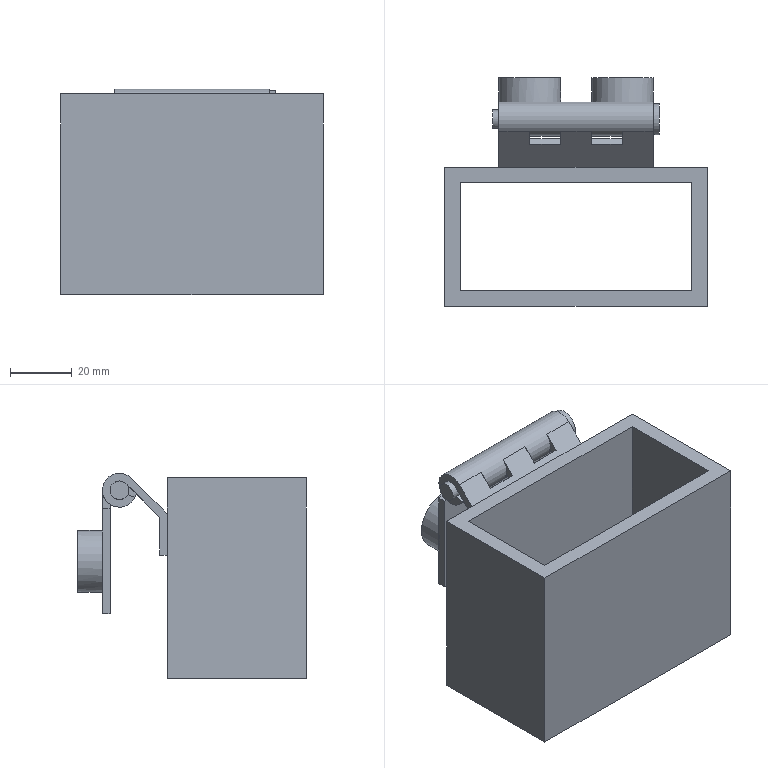Part | STEP file | 1 solid | 75 faces | box 85 x 74 x 66.5 mm | volume 93814 mm3 | plane 60 | cylinder 15 | commonest cylinder face diameters 8.5 x6 6 x5 20 x2 10 x1 11 x1